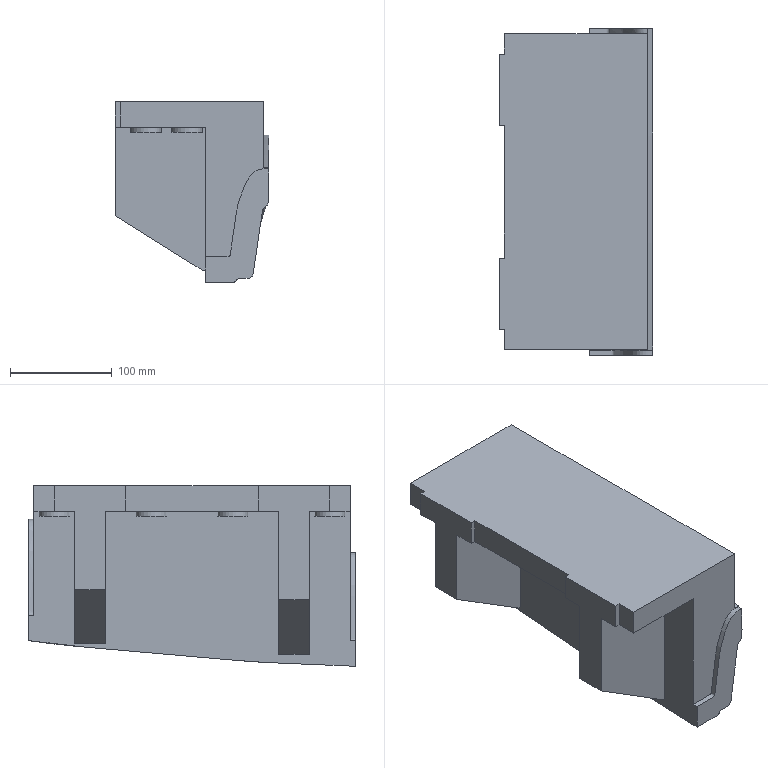Part | NX | features solid 2 | 1 solid | 125 faces | box 150.321 x 320 x 176.991 mm | volume 4128385 mm3 | spline 61 | plane 39 | cylinder 23 | sphere 2 | commonest cylinder face diameters 30 x6 10 x5 6.001 x4 6.007 x1 9 x1 9.001 x1